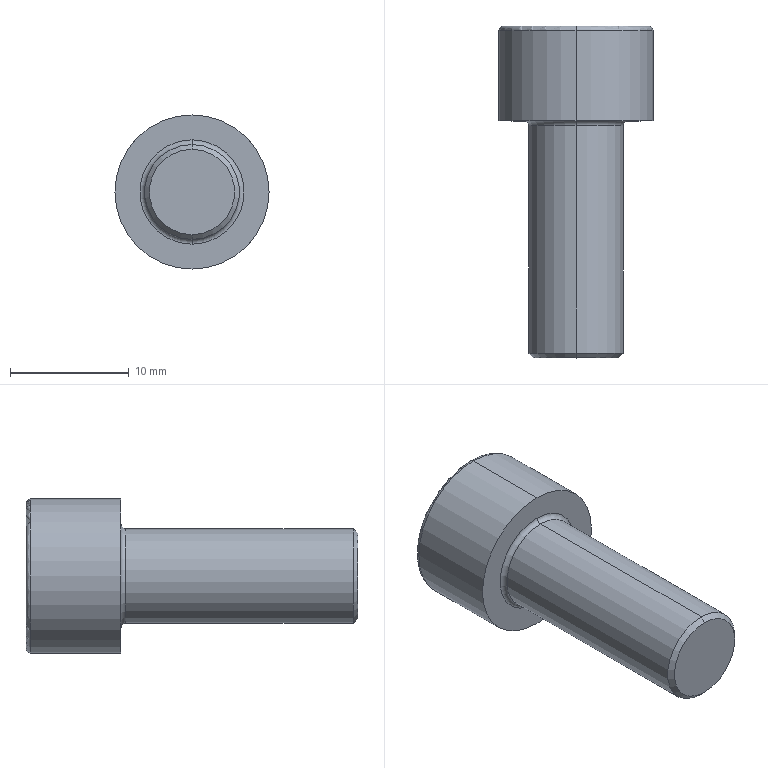Part | STEP file | 1 solid | 20 faces | box 13 x 28 x 13 mm | volume 1940 mm3 | plane 10 | torus 4 | cylinder 4 | cone 2 | commonest cylinder face diameters 8 x2 13 x2
STEP:
#1=CARTESIAN_POINT('',(0.,-20.,-3.6));
#2=VERTEX_POINT('',#1);
#3=CARTESIAN_POINT('',(0.,-20.,3.6));
#4=VERTEX_POINT('',#3);
#5=CARTESIAN_POINT('',(0.,-20.,0.));
#6=DIRECTION('',(0.,-1.,0.));
#7=DIRECTION('',(0.,0.,-1.));
#8=AXIS2_PLACEMENT_3D('',#5,#6,#7);
#9=CIRCLE('',#8,3.6);
#10=EDGE_CURVE('',#2,#4,#9,.T.);
#11=ORIENTED_EDGE('',*,*,#10,.F.);
#12=CARTESIAN_POINT('',(0.,-19.6,-4.));
#13=VERTEX_POINT('',#12);
#14=CARTESIAN_POINT('',(0.,-20.,-3.6));
#15=DIRECTION('',(0.,0.7071,-0.7071));
#16=VECTOR('',#15,1000.);
#17=LINE('',#14,#16);
#18=EDGE_CURVE('',#2,#13,#17,.T.);
#19=ORIENTED_EDGE('',*,*,#18,.T.);
#20=CARTESIAN_POINT('',(0.,-19.6,4.));
#21=VERTEX_POINT('',#20);
#22=CARTESIAN_POINT('',(0.,-19.6,0.));
#23=DIRECTION('',(0.,1.,0.));
#24=DIRECTION('',(0.,0.,-1.));
#25=AXIS2_PLACEMENT_3D('',#22,#23,#24);
#26=CIRCLE('',#25,4.);
#27=EDGE_CURVE('',#21,#13,#26,.T.);
#28=ORIENTED_EDGE('',*,*,#27,.F.);
#29=CARTESIAN_POINT('',(0.,-20.,3.6));
#30=DIRECTION('',(0.,0.7071,0.7071));
#31=VECTOR('',#30,1000.);
#32=LINE('',#29,#31);
#33=EDGE_CURVE('',#4,#21,#32,.T.);
#34=ORIENTED_EDGE('',*,*,#33,.F.);
#35=EDGE_LOOP('',(#11,#19,#28,#34));
#36=FACE_OUTER_BOUND('',#35,.T.);
#37=CARTESIAN_POINT('',(0.,-20.,0.));
#38=DIRECTION('',(0.,1.,0.));
#39=DIRECTION('',(0.,0.,1.));
#40=AXIS2_PLACEMENT_3D('',#37,#38,#39);
#41=CONICAL_SURFACE('',#40,3.6,0.7854);
#42=ADVANCED_FACE('',(#36),#41,.T.);
#43=CARTESIAN_POINT('',(0.,7.6,-6.5));
#44=VERTEX_POINT('',#43);
#45=CARTESIAN_POINT('',(0.,7.6,6.5));
#46=VERTEX_POINT('',#45);
#47=CARTESIAN_POINT('',(0.,7.6,0.));
#48=DIRECTION('',(0.,-1.,0.));
#49=DIRECTION('',(0.,0.,1.));
#50=AXIS2_PLACEMENT_3D('',#47,#48,#49);
#51=CIRCLE('',#50,6.5);
#52=EDGE_CURVE('',#44,#46,#51,.T.);
#53=ORIENTED_EDGE('',*,*,#52,.F.);
#54=CARTESIAN_POINT('',(0.,8.,-6.1));
#55=VERTEX_POINT('',#54);
#56=CARTESIAN_POINT('',(0.,7.6,-6.1));
#57=DIRECTION('',(1.,0.,0.));
#58=DIRECTION('',(0.,0.,-1.));
#59=AXIS2_PLACEMENT_3D('',#56,#57,#58);
#60=CIRCLE('',#59,0.4);
#61=EDGE_CURVE('',#44,#55,#60,.T.);
#62=ORIENTED_EDGE('',*,*,#61,.T.);
#63=CARTESIAN_POINT('',(0.,8.,6.1));
#64=VERTEX_POINT('',#63);
#65=CARTESIAN_POINT('',(0.,8.,0.));
#66=DIRECTION('',(0.,1.,0.));
#67=DIRECTION('',(0.,0.,1.));
#68=AXIS2_PLACEMENT_3D('',#65,#66,#67);
#69=CIRCLE('',#68,6.1);
#70=EDGE_CURVE('',#64,#55,#69,.T.);
#71=ORIENTED_EDGE('',*,*,#70,.F.);
#72=CARTESIAN_POINT('',(0.,7.6,6.1));
#73=DIRECTION('',(-1.,0.,0.));
#74=DIRECTION('',(0.,0.,1.));
#75=AXIS2_PLACEMENT_3D('',#72,#73,#74);
#76=CIRCLE('',#75,0.4);
#77=EDGE_CURVE('',#46,#64,#76,.T.);
#78=ORIENTED_EDGE('',*,*,#77,.F.);
#79=EDGE_LOOP('',(#53,#62,#71,#78));
#80=FACE_OUTER_BOUND('',#79,.T.);
#81=CARTESIAN_POINT('',(0.,7.6,0.));
#82=DIRECTION('',(0.,1.,0.));
#83=DIRECTION('',(0.,0.,1.));
#84=AXIS2_PLACEMENT_3D('',#81,#82,#83);
#85=TOROIDAL_SURFACE('',#84,6.1,0.4);
#86=ADVANCED_FACE('',(#80),#85,.T.);
#87=CARTESIAN_POINT('',(0.,-0.4,4.));
#88=VERTEX_POINT('',#87);
#89=CARTESIAN_POINT('',(0.,-0.4,-4.));
#90=VERTEX_POINT('',#89);
#91=CARTESIAN_POINT('',(0.,-0.4,0.));
#92=DIRECTION('',(0.,-1.,0.));
#93=DIRECTION('',(0.,0.,-1.));
#94=AXIS2_PLACEMENT_3D('',#91,#92,#93);
#95=CIRCLE('',#94,4.);
#96=EDGE_CURVE('',#88,#90,#95,.T.);
#97=ORIENTED_EDGE('',*,*,#96,.F.);
#98=CARTESIAN_POINT('',(0.,0.,4.4));
#99=VERTEX_POINT('',#98);
#100=CARTESIAN_POINT('',(0.,-0.4,4.4));
#101=DIRECTION('',(1.,0.,0.));
#102=DIRECTION('',(0.,0.,-1.));
#103=AXIS2_PLACEMENT_3D('',#100,#101,#102);
#104=CIRCLE('',#103,0.4);
#105=EDGE_CURVE('',#88,#99,#104,.T.);
#106=ORIENTED_EDGE('',*,*,#105,.T.);
#107=CARTESIAN_POINT('',(0.,0.,-4.4));
#108=VERTEX_POINT('',#107);
#109=CARTESIAN_POINT('',(0.,0.,0.));
#110=DIRECTION('',(0.,1.,0.));
#111=DIRECTION('',(0.,0.,-1.));
#112=AXIS2_PLACEMENT_3D('',#109,#110,#111);
#113=CIRCLE('',#112,4.4);
#114=EDGE_CURVE('',#108,#99,#113,.T.);
#115=ORIENTED_EDGE('',*,*,#114,.F.);
#116=CARTESIAN_POINT('',(0.,-0.4,-4.4));
#117=DIRECTION('',(-1.,0.,0.));
#118=DIRECTION('',(0.,0.,1.));
#119=AXIS2_PLACEMENT_3D('',#116,#117,#118);
#120=CIRCLE('',#119,0.4);
#121=EDGE_CURVE('',#90,#108,#120,.T.);
#122=ORIENTED_EDGE('',*,*,#121,.F.);
#123=EDGE_LOOP('',(#97,#106,#115,#122));
#124=FACE_OUTER_BOUND('',#123,.T.);
#125=CARTESIAN_POINT('',(0.,-0.4,0.));
#126=DIRECTION('',(0.,-1.,0.));
#127=DIRECTION('',(0.,0.,-1.));
#128=AXIS2_PLACEMENT_3D('',#125,#126,#127);
#129=TOROIDAL_SURFACE('',#128,4.4,0.4);
#130=ADVANCED_FACE('',(#124),#129,.F.);
#131=CARTESIAN_POINT('',(0.,-0.4,0.));
#132=DIRECTION('',(0.,-1.,0.));
#133=DIRECTION('',(0.,0.,-1.));
#134=AXIS2_PLACEMENT_3D('',#131,#132,#133);
#135=CIRCLE('',#134,4.);
#136=EDGE_CURVE('',#90,#88,#135,.T.);
#137=ORIENTED_EDGE('',*,*,#136,.T.);
#138=CARTESIAN_POINT('',(0.,0.,4.));
#139=DIRECTION('',(0.,-1.,0.));
#140=VECTOR('',#139,1000.);
#141=LINE('',#138,#140);
#142=EDGE_CURVE('',#88,#21,#141,.T.);
#143=ORIENTED_EDGE('',*,*,#142,.T.);
#144=ORIENTED_EDGE('',*,*,#27,.T.);
#145=CARTESIAN_POINT('',(0.,0.,-4.));
#146=DIRECTION('',(0.,-1.,0.));
#147=VECTOR('',#146,1000.);
#148=LINE('',#145,#147);
#149=EDGE_CURVE('',#90,#13,#148,.T.);
#150=ORIENTED_EDGE('',*,*,#149,.F.);
#151=EDGE_LOOP('',(#137,#143,#144,#150));
#152=FACE_OUTER_BOUND('',#151,.T.);
#153=CARTESIAN_POINT('',(0.,0.,0.));
#154=DIRECTION('',(0.,-1.,0.));
#155=DIRECTION('',(0.,0.,-1.));
#156=AXIS2_PLACEMENT_3D('',#153,#154,#155);
#157=CYLINDRICAL_SURFACE('',#156,4.);
#158=ADVANCED_FACE('',(#152),#157,.T.);
#159=ORIENTED_EDGE('',*,*,#52,.T.);
#160=CARTESIAN_POINT('',(0.,0.,6.5));
#161=VERTEX_POINT('',#160);
#162=CARTESIAN_POINT('',(0.,0.,6.5));
#163=DIRECTION('',(0.,-1.,0.));
#164=VECTOR('',#163,1000.);
#165=LINE('',#162,#164);
#166=EDGE_CURVE('',#46,#161,#165,.T.);
#167=ORIENTED_EDGE('',*,*,#166,.T.);
#168=CARTESIAN_POINT('',(0.,0.,-6.5));
#169=VERTEX_POINT('',#168);
#170=CARTESIAN_POINT('',(0.,0.,0.));
#171=DIRECTION('',(0.,-1.,0.));
#172=DIRECTION('',(0.,0.,-1.));
#173=AXIS2_PLACEMENT_3D('',#170,#171,#172);
#174=CIRCLE('',#173,6.5);
#175=EDGE_CURVE('',#169,#161,#174,.T.);
#176=ORIENTED_EDGE('',*,*,#175,.F.);
#177=CARTESIAN_POINT('',(0.,0.,-6.5));
#178=DIRECTION('',(0.,-1.,0.));
#179=VECTOR('',#178,1000.);
#180=LINE('',#177,#179);
#181=EDGE_CURVE('',#44,#169,#180,.T.);
#182=ORIENTED_EDGE('',*,*,#181,.F.);
#183=EDGE_LOOP('',(#159,#167,#176,#182));
#184=FACE_OUTER_BOUND('',#183,.T.);
#185=CARTESIAN_POINT('',(0.,0.,0.));
#186=DIRECTION('',(0.,-1.,0.));
#187=DIRECTION('',(0.,0.,-1.));
#188=AXIS2_PLACEMENT_3D('',#185,#186,#187);
#189=CYLINDRICAL_SURFACE('',#188,6.5);
#190=ADVANCED_FACE('',(#184),#189,.T.);
#191=ORIENTED_EDGE('',*,*,#70,.T.);
#192=CARTESIAN_POINT('',(0.,8.,0.));
#193=DIRECTION('',(0.,1.,0.));
#194=DIRECTION('',(0.,0.,1.));
#195=AXIS2_PLACEMENT_3D('',#192,#193,#194);
#196=CIRCLE('',#195,6.1);
#197=EDGE_CURVE('',#55,#64,#196,.T.);
#198=ORIENTED_EDGE('',*,*,#197,.T.);
#199=EDGE_LOOP('',(#191,#198));
#200=FACE_OUTER_BOUND('',#199,.T.);
#201=CARTESIAN_POINT('',(0.,8.,-3.464));
#202=VERTEX_POINT('',#201);
#203=CARTESIAN_POINT('',(-3.,8.,-1.732));
#204=VERTEX_POINT('',#203);
#205=CARTESIAN_POINT('',(0.,8.,-3.464));
#206=DIRECTION('',(-0.866,0.,0.5));
#207=VECTOR('',#206,1000.);
#208=LINE('',#205,#207);
#209=EDGE_CURVE('',#202,#204,#208,.T.);
#210=ORIENTED_EDGE('',*,*,#209,.F.);
#211=CARTESIAN_POINT('',(3.,8.,-1.732));
#212=VERTEX_POINT('',#211);
#213=CARTESIAN_POINT('',(3.,8.,-1.732));
#214=DIRECTION('',(-0.866,0.,-0.5));
#215=VECTOR('',#214,1000.);
#216=LINE('',#213,#215);
#217=EDGE_CURVE('',#212,#202,#216,.T.);
#218=ORIENTED_EDGE('',*,*,#217,.F.);
#219=CARTESIAN_POINT('',(3.,8.,1.732));
#220=VERTEX_POINT('',#219);
#221=CARTESIAN_POINT('',(3.,8.,1.732));
#222=DIRECTION('',(0.,0.,-1.));
#223=VECTOR('',#222,1000.);
#224=LINE('',#221,#223);
#225=EDGE_CURVE('',#220,#212,#224,.T.);
#226=ORIENTED_EDGE('',*,*,#225,.F.);
#227=CARTESIAN_POINT('',(0.,8.,3.464));
#228=VERTEX_POINT('',#227);
#229=CARTESIAN_POINT('',(0.,8.,3.464));
#230=DIRECTION('',(0.866,0.,-0.5));
#231=VECTOR('',#230,1000.);
#232=LINE('',#229,#231);
#233=EDGE_CURVE('',#228,#220,#232,.T.);
#234=ORIENTED_EDGE('',*,*,#233,.F.);
#235=CARTESIAN_POINT('',(-3.,8.,1.732));
#236=VERTEX_POINT('',#235);
#237=CARTESIAN_POINT('',(-3.,8.,1.732));
#238=DIRECTION('',(0.866,0.,0.5));
#239=VECTOR('',#238,1000.);
#240=LINE('',#237,#239);
#241=EDGE_CURVE('',#236,#228,#240,.T.);
#242=ORIENTED_EDGE('',*,*,#241,.F.);
#243=CARTESIAN_POINT('',(-3.,8.,-1.732));
#244=DIRECTION('',(0.,0.,1.));
#245=VECTOR('',#244,1000.);
#246=LINE('',#243,#245);
#247=EDGE_CURVE('',#204,#236,#246,.T.);
#248=ORIENTED_EDGE('',*,*,#247,.F.);
#249=EDGE_LOOP('',(#210,#218,#226,#234,#242,#248));
#250=FACE_BOUND('',#249,.T.);
#251=CARTESIAN_POINT('',(0.,8.,0.));
#252=DIRECTION('',(0.,1.,0.));
#253=DIRECTION('',(0.,0.,1.));
#254=AXIS2_PLACEMENT_3D('',#251,#252,#253);
#255=PLANE('',#254);
#256=ADVANCED_FACE('',(#200,#250),#255,.T.);
#257=ORIENTED_EDGE('',*,*,#166,.F.);
#258=CARTESIAN_POINT('',(0.,7.6,0.));
#259=DIRECTION('',(0.,-1.,0.));
#260=DIRECTION('',(0.,0.,1.));
#261=AXIS2_PLACEMENT_3D('',#258,#259,#260);
#262=CIRCLE('',#261,6.5);
#263=EDGE_CURVE('',#46,#44,#262,.T.);
#264=ORIENTED_EDGE('',*,*,#263,.T.);
#265=ORIENTED_EDGE('',*,*,#181,.T.);
#266=CARTESIAN_POINT('',(0.,0.,0.));
#267=DIRECTION('',(0.,-1.,0.));
#268=DIRECTION('',(0.,0.,-1.));
#269=AXIS2_PLACEMENT_3D('',#266,#267,#268);
#270=CIRCLE('',#269,6.5);
#271=EDGE_CURVE('',#161,#169,#270,.T.);
#272=ORIENTED_EDGE('',*,*,#271,.F.);
#273=EDGE_LOOP('',(#257,#264,#265,#272));
#274=FACE_OUTER_BOUND('',#273,.T.);
#275=CARTESIAN_POINT('',(0.,0.,0.));
#276=DIRECTION('',(0.,-1.,0.));
#277=DIRECTION('',(0.,0.,-1.));
#278=AXIS2_PLACEMENT_3D('',#275,#276,#277);
#279=CYLINDRICAL_SURFACE('',#278,6.5);
#280=ADVANCED_FACE('',(#274),#279,.T.);
#281=ORIENTED_EDGE('',*,*,#114,.T.);
#282=CARTESIAN_POINT('',(0.,0.,0.));
#283=DIRECTION('',(0.,1.,0.));
#284=DIRECTION('',(0.,0.,-1.));
#285=AXIS2_PLACEMENT_3D('',#282,#283,#284);
#286=CIRCLE('',#285,4.4);
#287=EDGE_CURVE('',#99,#108,#286,.T.);
#288=ORIENTED_EDGE('',*,*,#287,.T.);
#289=EDGE_LOOP('',(#281,#288));
#290=FACE_BOUND('',#289,.T.);
#291=ORIENTED_EDGE('',*,*,#175,.T.);
#292=ORIENTED_EDGE('',*,*,#271,.T.);
#293=EDGE_LOOP('',(#291,#292));
#294=FACE_OUTER_BOUND('',#293,.T.);
#295=CARTESIAN_POINT('',(6.5,0.,0.));
#296=DIRECTION('',(0.,-1.,0.));
#297=DIRECTION('',(0.,0.,-1.));
#298=AXIS2_PLACEMENT_3D('',#295,#296,#297);
#299=PLANE('',#298);
#300=ADVANCED_FACE('',(#290,#294),#299,.T.);
#301=ORIENTED_EDGE('',*,*,#142,.F.);
#302=ORIENTED_EDGE('',*,*,#96,.T.);
#303=ORIENTED_EDGE('',*,*,#149,.T.);
#304=CARTESIAN_POINT('',(0.,-19.6,0.));
#305=DIRECTION('',(0.,1.,0.));
#306=DIRECTION('',(0.,0.,-1.));
#307=AXIS2_PLACEMENT_3D('',#304,#305,#306);
#308=CIRCLE('',#307,4.);
#309=EDGE_CURVE('',#13,#21,#308,.T.);
#310=ORIENTED_EDGE('',*,*,#309,.T.);
#311=EDGE_LOOP('',(#301,#302,#303,#310));
#312=FACE_OUTER_BOUND('',#311,.T.);
#313=CARTESIAN_POINT('',(0.,0.,0.));
#314=DIRECTION('',(0.,-1.,0.));
#315=DIRECTION('',(0.,0.,-1.));
#316=AXIS2_PLACEMENT_3D('',#313,#314,#315);
#317=CYLINDRICAL_SURFACE('',#316,4.);
#318=ADVANCED_FACE('',(#312),#317,.T.);
#319=CARTESIAN_POINT('',(0.,-20.,0.));
#320=DIRECTION('',(0.,-1.,0.));
#321=DIRECTION('',(0.,0.,-1.));
#322=AXIS2_PLACEMENT_3D('',#319,#320,#321);
#323=CIRCLE('',#322,3.6);
#324=EDGE_CURVE('',#4,#2,#323,.T.);
#325=ORIENTED_EDGE('',*,*,#324,.T.);
#326=ORIENTED_EDGE('',*,*,#10,.T.);
#327=EDGE_LOOP('',(#325,#326));
#328=FACE_OUTER_BOUND('',#327,.T.);
#329=CARTESIAN_POINT('',(4.,-20.,0.));
#330=DIRECTION('',(0.,-1.,0.));
#331=DIRECTION('',(0.,0.,-1.));
#332=AXIS2_PLACEMENT_3D('',#329,#330,#331);
#333=PLANE('',#332);
#334=ADVANCED_FACE('',(#328),#333,.T.);
#335=ORIENTED_EDGE('',*,*,#209,.T.);
#336=CARTESIAN_POINT('',(-3.,4.,-1.732));
#337=VERTEX_POINT('',#336);
#338=CARTESIAN_POINT('',(-3.,4.,-1.732));
#339=DIRECTION('',(0.,1.,0.));
#340=VECTOR('',#339,1000.);
#341=LINE('',#338,#340);
#342=EDGE_CURVE('',#337,#204,#341,.T.);
#343=ORIENTED_EDGE('',*,*,#342,.F.);
#344=CARTESIAN_POINT('',(0.,4.,-3.464));
#345=VERTEX_POINT('',#344);
#346=CARTESIAN_POINT('',(0.,4.,-3.464));
#347=DIRECTION('',(-0.866,0.,0.5));
#348=VECTOR('',#347,1000.);
#349=LINE('',#346,#348);
#350=EDGE_CURVE('',#345,#337,#349,.T.);
#351=ORIENTED_EDGE('',*,*,#350,.F.);
#352=CARTESIAN_POINT('',(0.,4.,-3.464));
#353=DIRECTION('',(0.,1.,0.));
#354=VECTOR('',#353,1000.);
#355=LINE('',#352,#354);
#356=EDGE_CURVE('',#345,#202,#355,.T.);
#357=ORIENTED_EDGE('',*,*,#356,.T.);
#358=EDGE_LOOP('',(#335,#343,#351,#357));
#359=FACE_OUTER_BOUND('',#358,.T.);
#360=CARTESIAN_POINT('',(0.,4.,-3.464));
#361=DIRECTION('',(-0.5,0.,-0.866));
#362=DIRECTION('',(-0.866,0.,0.5));
#363=AXIS2_PLACEMENT_3D('',#360,#361,#362);
#364=PLANE('',#363);
#365=ADVANCED_FACE('',(#359),#364,.F.);
#366=ORIENTED_EDGE('',*,*,#217,.T.);
#367=ORIENTED_EDGE('',*,*,#356,.F.);
#368=CARTESIAN_POINT('',(3.,4.,-1.732));
#369=VERTEX_POINT('',#368);
#370=CARTESIAN_POINT('',(3.,4.,-1.732));
#371=DIRECTION('',(-0.866,0.,-0.5));
#372=VECTOR('',#371,1000.);
#373=LINE('',#370,#372);
#374=EDGE_CURVE('',#369,#345,#373,.T.);
#375=ORIENTED_EDGE('',*,*,#374,.F.);
#376=CARTESIAN_POINT('',(3.,4.,-1.732));
#377=DIRECTION('',(0.,1.,0.));
#378=VECTOR('',#377,1000.);
#379=LINE('',#376,#378);
#380=EDGE_CURVE('',#369,#212,#379,.T.);
#381=ORIENTED_EDGE('',*,*,#380,.T.);
#382=EDGE_LOOP('',(#366,#367,#375,#381));
#383=FACE_OUTER_BOUND('',#382,.T.);
#384=CARTESIAN_POINT('',(3.,4.,-1.732));
#385=DIRECTION('',(0.5,0.,-0.866));
#386=DIRECTION('',(-0.866,0.,-0.5));
#387=AXIS2_PLACEMENT_3D('',#384,#385,#386);
#388=PLANE('',#387);
#389=ADVANCED_FACE('',(#383),#388,.F.);
#390=ORIENTED_EDGE('',*,*,#225,.T.);
#391=ORIENTED_EDGE('',*,*,#380,.F.);
#392=CARTESIAN_POINT('',(3.,4.,1.732));
#393=VERTEX_POINT('',#392);
#394=CARTESIAN_POINT('',(3.,4.,1.732));
#395=DIRECTION('',(0.,0.,-1.));
#396=VECTOR('',#395,1000.);
#397=LINE('',#394,#396);
#398=EDGE_CURVE('',#393,#369,#397,.T.);
#399=ORIENTED_EDGE('',*,*,#398,.F.);
#400=CARTESIAN_POINT('',(3.,4.,1.732));
#401=DIRECTION('',(0.,1.,0.));
#402=VECTOR('',#401,1000.);
#403=LINE('',#400,#402);
#404=EDGE_CURVE('',#393,#220,#403,.T.);
#405=ORIENTED_EDGE('',*,*,#404,.T.);
#406=EDGE_LOOP('',(#390,#391,#399,#405));
#407=FACE_OUTER_BOUND('',#406,.T.);
#408=CARTESIAN_POINT('',(3.,4.,1.732));
#409=DIRECTION('',(1.,0.,0.));
#410=DIRECTION('',(0.,0.,-1.));
#411=AXIS2_PLACEMENT_3D('',#408,#409,#410);
#412=PLANE('',#411);
#413=ADVANCED_FACE('',(#407),#412,.F.);
#414=ORIENTED_EDGE('',*,*,#233,.T.);
#415=ORIENTED_EDGE('',*,*,#404,.F.);
#416=CARTESIAN_POINT('',(0.,4.,3.464));
#417=VERTEX_POINT('',#416);
#418=CARTESIAN_POINT('',(0.,4.,3.464));
#419=DIRECTION('',(0.866,0.,-0.5));
#420=VECTOR('',#419,1000.);
#421=LINE('',#418,#420);
#422=EDGE_CURVE('',#417,#393,#421,.T.);
#423=ORIENTED_EDGE('',*,*,#422,.F.);
#424=CARTESIAN_POINT('',(0.,4.,3.464));
#425=DIRECTION('',(0.,1.,0.));
#426=VECTOR('',#425,1000.);
#427=LINE('',#424,#426);
#428=EDGE_CURVE('',#417,#228,#427,.T.);
#429=ORIENTED_EDGE('',*,*,#428,.T.);
#430=EDGE_LOOP('',(#414,#415,#423,#429));
#431=FACE_OUTER_BOUND('',#430,.T.);
#432=CARTESIAN_POINT('',(0.,4.,3.464));
#433=DIRECTION('',(0.5,0.,0.866));
#434=DIRECTION('',(0.866,0.,-0.5));
#435=AXIS2_PLACEMENT_3D('',#432,#433,#434);
#436=PLANE('',#435);
#437=ADVANCED_FACE('',(#431),#436,.F.);
#438=ORIENTED_EDGE('',*,*,#241,.T.);
#439=ORIENTED_EDGE('',*,*,#428,.F.);
#440=CARTESIAN_POINT('',(-3.,4.,1.732));
#441=VERTEX_POINT('',#440);
#442=CARTESIAN_POINT('',(-3.,4.,1.732));
#443=DIRECTION('',(0.866,0.,0.5));
#444=VECTOR('',#443,1000.);
#445=LINE('',#442,#444);
#446=EDGE_CURVE('',#441,#417,#445,.T.);
#447=ORIENTED_EDGE('',*,*,#446,.F.);
#448=CARTESIAN_POINT('',(-3.,4.,1.732));
#449=DIRECTION('',(0.,1.,0.));
#450=VECTOR('',#449,1000.);
#451=LINE('',#448,#450);
#452=EDGE_CURVE('',#441,#236,#451,.T.);
#453=ORIENTED_EDGE('',*,*,#452,.T.);
#454=EDGE_LOOP('',(#438,#439,#447,#453));
#455=FACE_OUTER_BOUND('',#454,.T.);
#456=CARTESIAN_POINT('',(-3.,4.,1.732));
#457=DIRECTION('',(-0.5,0.,0.866));
#458=DIRECTION('',(0.866,0.,0.5));
#459=AXIS2_PLACEMENT_3D('',#456,#457,#458);
#460=PLANE('',#459);
#461=ADVANCED_FACE('',(#455),#460,.F.);
#462=ORIENTED_EDGE('',*,*,#247,.T.);
#463=ORIENTED_EDGE('',*,*,#452,.F.);
#464=CARTESIAN_POINT('',(-3.,4.,-1.732));
#465=DIRECTION('',(0.,0.,1.));
#466=VECTOR('',#465,1000.);
#467=LINE('',#464,#466);
#468=EDGE_CURVE('',#337,#441,#467,.T.);
#469=ORIENTED_EDGE('',*,*,#468,.F.);
#470=ORIENTED_EDGE('',*,*,#342,.T.);
#471=EDGE_LOOP('',(#462,#463,#469,#470));
#472=FACE_OUTER_BOUND('',#471,.T.);
#473=CARTESIAN_POINT('',(-3.,4.,-1.732));
#474=DIRECTION('',(-1.,0.,0.));
#475=DIRECTION('',(0.,0.,1.));
#476=AXIS2_PLACEMENT_3D('',#473,#474,#475);
#477=PLANE('',#476);
#478=ADVANCED_FACE('',(#472),#477,.F.);
#479=ORIENTED_EDGE('',*,*,#350,.T.);
#480=ORIENTED_EDGE('',*,*,#468,.T.);
#481=ORIENTED_EDGE('',*,*,#446,.T.);
#482=ORIENTED_EDGE('',*,*,#422,.T.);
#483=ORIENTED_EDGE('',*,*,#398,.T.);
#484=ORIENTED_EDGE('',*,*,#374,.T.);
#485=EDGE_LOOP('',(#479,#480,#481,#482,#483,#484));
#486=FACE_OUTER_BOUND('',#485,.T.);
#487=CARTESIAN_POINT('',(0.,4.,0.));
#488=DIRECTION('',(0.,1.,0.));
#489=DIRECTION('',(0.,0.,1.));
#490=AXIS2_PLACEMENT_3D('',#487,#488,#489);
#491=PLANE('',#490);
#492=ADVANCED_FACE('',(#486),#491,.T.);
#493=ORIENTED_EDGE('',*,*,#105,.F.);
#494=ORIENTED_EDGE('',*,*,#136,.F.);
#495=ORIENTED_EDGE('',*,*,#121,.T.);
#496=ORIENTED_EDGE('',*,*,#287,.F.);
#497=EDGE_LOOP('',(#493,#494,#495,#496));
#498=FACE_OUTER_BOUND('',#497,.T.);
#499=CARTESIAN_POINT('',(0.,-0.4,0.));
#500=DIRECTION('',(0.,-1.,0.));
#501=DIRECTION('',(0.,0.,-1.));
#502=AXIS2_PLACEMENT_3D('',#499,#500,#501);
#503=TOROIDAL_SURFACE('',#502,4.4,0.4);
#504=ADVANCED_FACE('',(#498),#503,.F.);
#505=ORIENTED_EDGE('',*,*,#61,.F.);
#506=ORIENTED_EDGE('',*,*,#263,.F.);
#507=ORIENTED_EDGE('',*,*,#77,.T.);
#508=ORIENTED_EDGE('',*,*,#197,.F.);
#509=EDGE_LOOP('',(#505,#506,#507,#508));
#510=FACE_OUTER_BOUND('',#509,.T.);
#511=CARTESIAN_POINT('',(0.,7.6,0.));
#512=DIRECTION('',(0.,1.,0.));
#513=DIRECTION('',(0.,0.,1.));
#514=AXIS2_PLACEMENT_3D('',#511,#512,#513);
#515=TOROIDAL_SURFACE('',#514,6.1,0.4);
#516=ADVANCED_FACE('',(#510),#515,.T.);
#517=ORIENTED_EDGE('',*,*,#18,.F.);
#518=ORIENTED_EDGE('',*,*,#324,.F.);
#519=ORIENTED_EDGE('',*,*,#33,.T.);
#520=ORIENTED_EDGE('',*,*,#309,.F.);
#521=EDGE_LOOP('',(#517,#518,#519,#520));
#522=FACE_OUTER_BOUND('',#521,.T.);
#523=CARTESIAN_POINT('',(0.,-20.,0.));
#524=DIRECTION('',(0.,1.,0.));
#525=DIRECTION('',(0.,0.,1.));
#526=AXIS2_PLACEMENT_3D('',#523,#524,#525);
#527=CONICAL_SURFACE('',#526,3.6,0.7854);
#528=ADVANCED_FACE('',(#522),#527,.T.);
#529=CLOSED_SHELL('',(#42,#86,#130,#158,#190,#256,#280,#300,#318,#334,#365,#389,#413,#437,#461,#478,#492,#504,#516,#528));
#530=MANIFOLD_SOLID_BREP('',#529);
#531=CARTESIAN_POINT('',(0.,0.,0.));
#532=DIRECTION('',(0.,0.,1.));
#533=DIRECTION('',(1.,0.,0.));
#534=AXIS2_PLACEMENT_3D('',#531,#532,#533);
#535=(LENGTH_UNIT()NAMED_UNIT(*)SI_UNIT(.MILLI.,.METRE.));
#536=UNCERTAINTY_MEASURE_WITH_UNIT(LENGTH_MEASURE(0.00001),#535,'','');
#537=(NAMED_UNIT(*)PLANE_ANGLE_UNIT()SI_UNIT($,.RADIAN.));
#538=(NAMED_UNIT(*)SI_UNIT($,.STERADIAN.)SOLID_ANGLE_UNIT());
#539=(GEOMETRIC_REPRESENTATION_CONTEXT(3)GLOBAL_UNCERTAINTY_ASSIGNED_CONTEXT((#536))GLOBAL_UNIT_ASSIGNED_CONTEXT((#535,#537,#538))REPRESENTATION_CONTEXT('',''));
#540=ADVANCED_BREP_SHAPE_REPRESENTATION('',(#530,#534),#539);